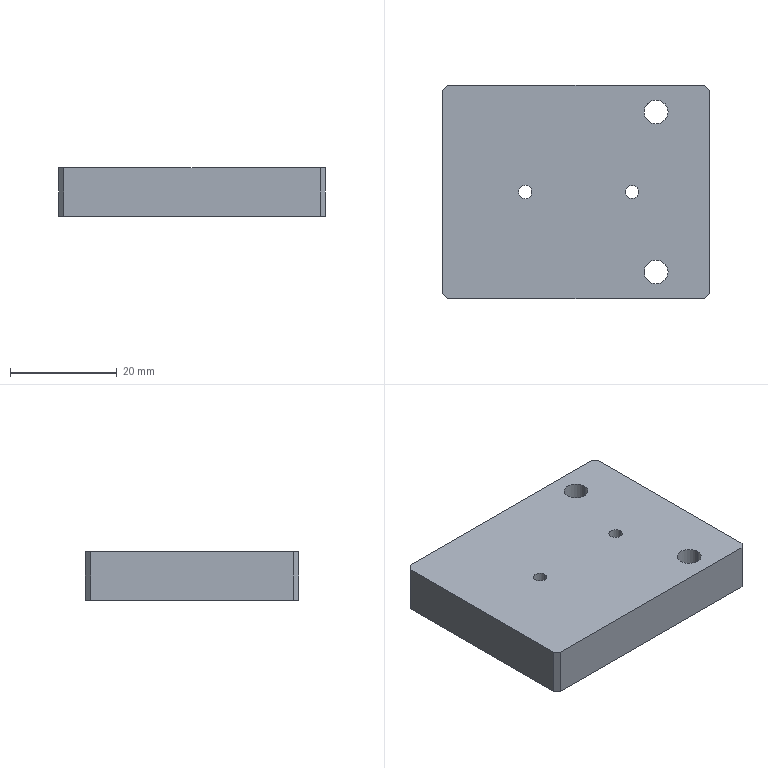Part | STEP file | PN_0028 Mount electronic clip mounting plate 3 | 1 solid | 24 faces | box 50 x 40 x 9 mm | volume 17291 mm3 | cylinder 12 | plane 12 | commonest cylinder face diameters 2.5 x4 4.5 x4 8 x4